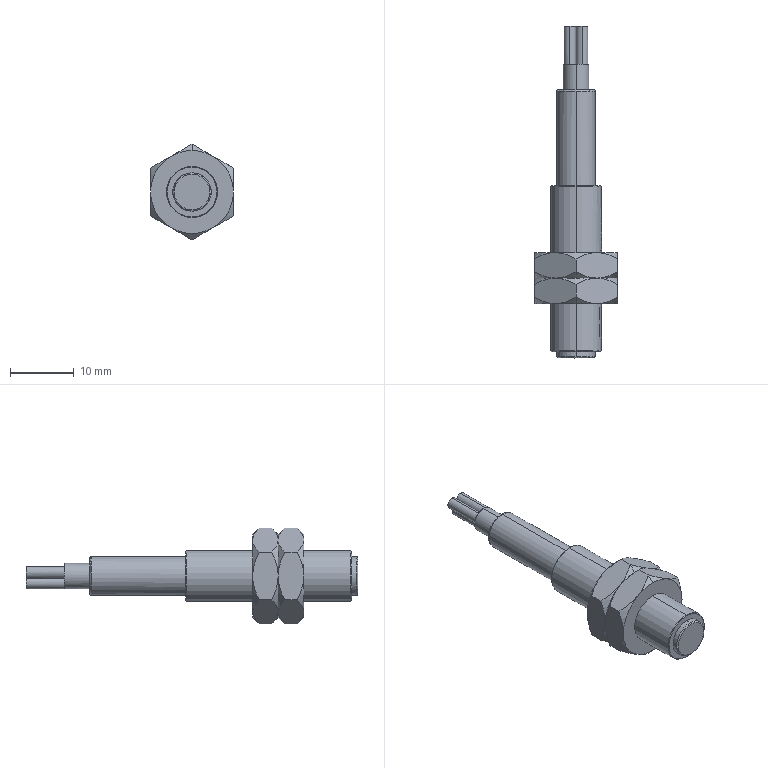Part | STEP file | 1 solid | 318 faces | box 13 x 52 x 15.011 mm | volume 2605 mm3 | plane 152 | spline 97 | cylinder 33 | cone 32 | torus 4 | commonest cylinder face diameters 8 x21 1.8 x6 6 x4 4 x2